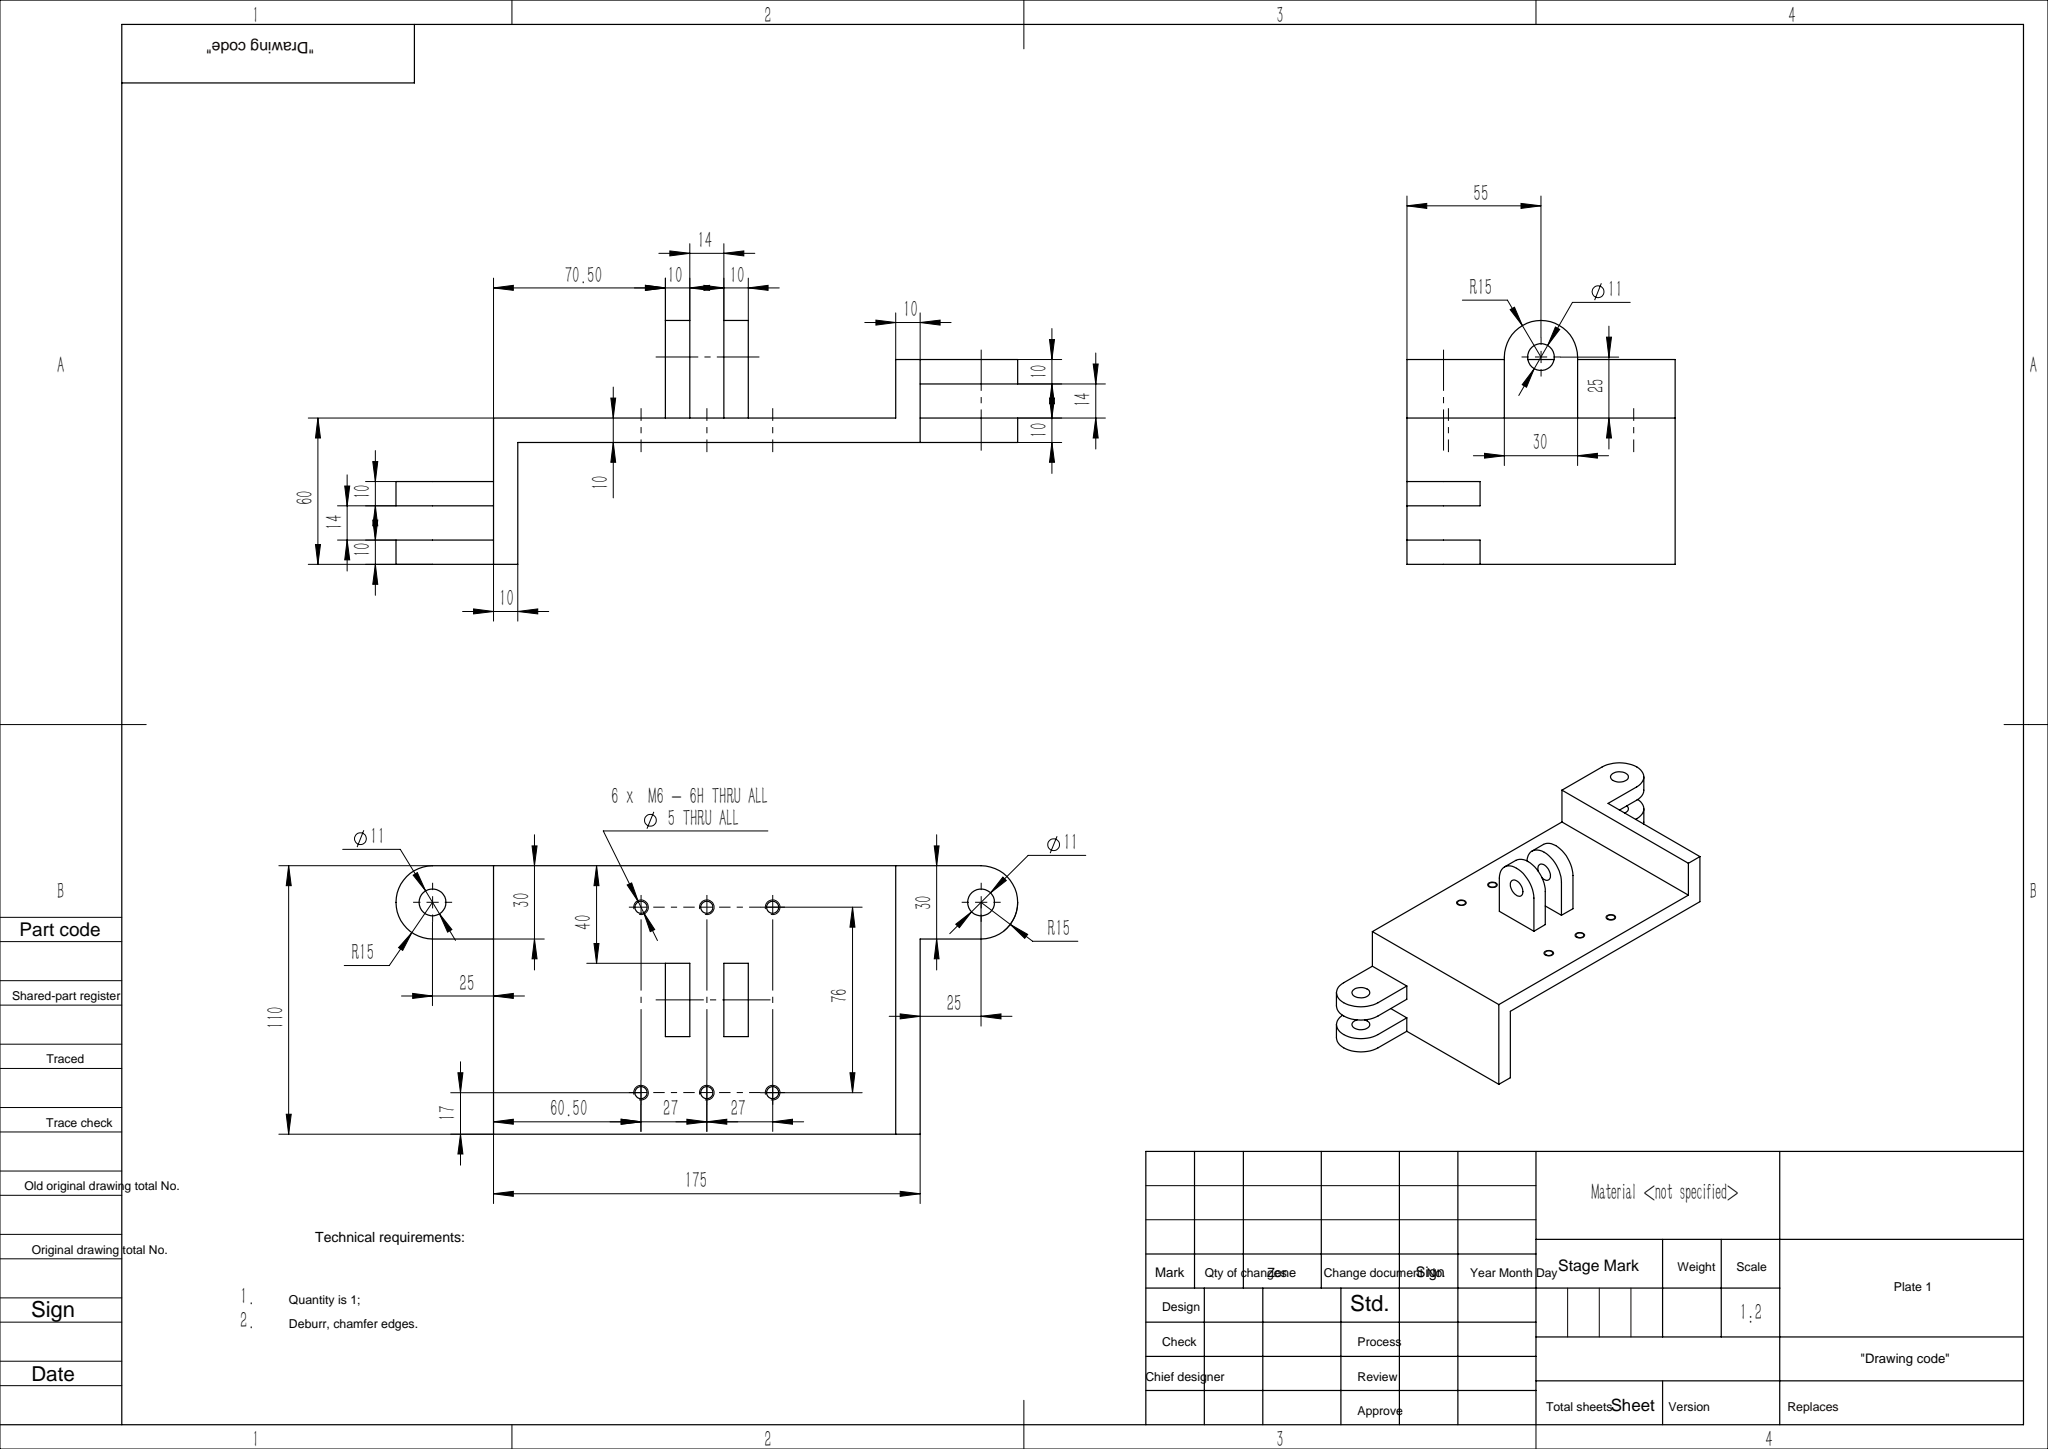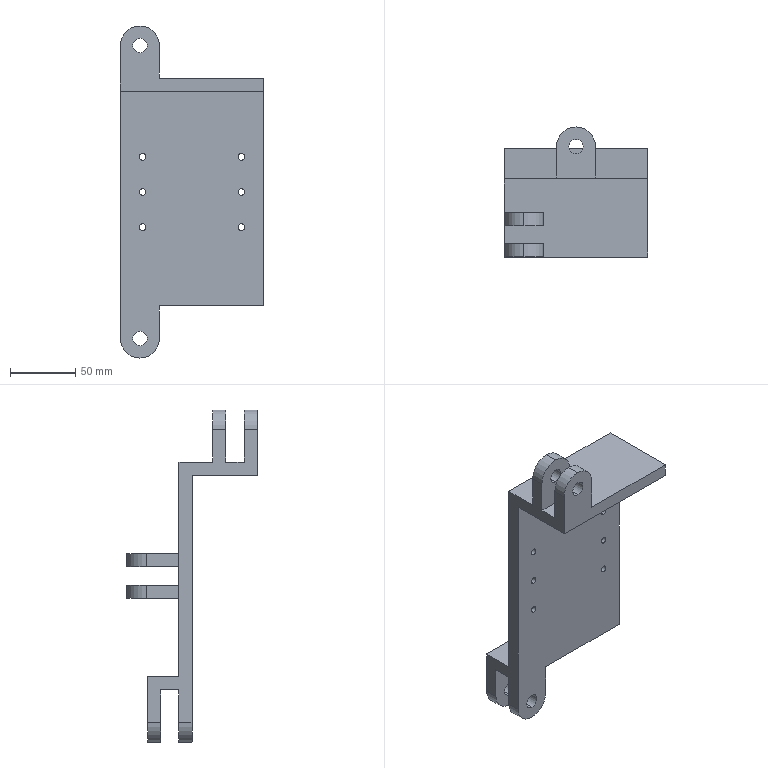Part | SolidWorks | features ICE 7, Fillet 3, LPattern 3, Extrusion 1, HoleWzd 1 | 1 solid | 63 faces | box 110 x 100 x 255 mm | volume 333226 mm3 | cylinder 36 | plane 27 | commonest cylinder face diameters 5 x12 11 x12 30 x12